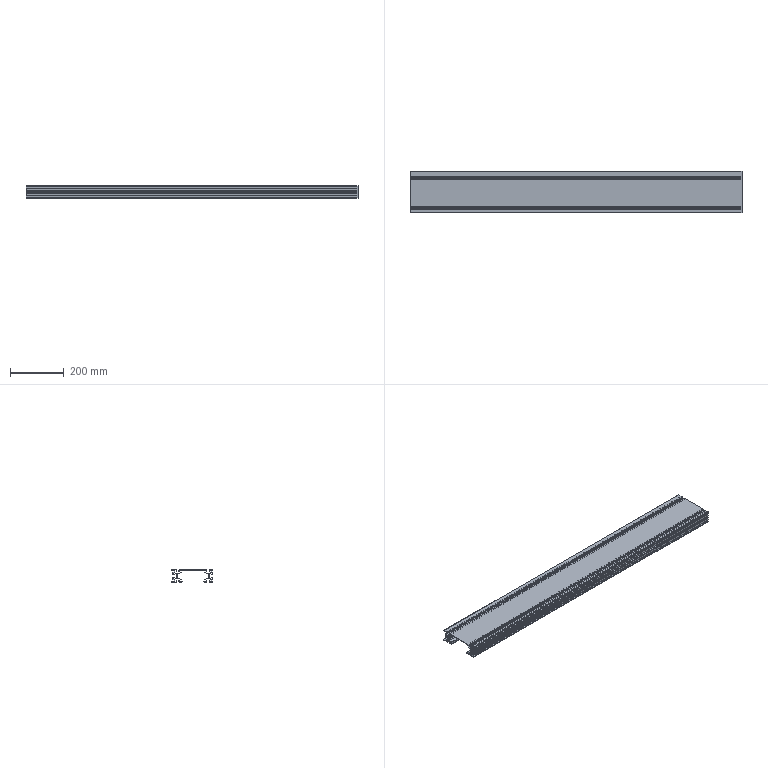Part | SolidWorks | features BaseBody 1 | 1 solid | 184 faces | box 1230 x 155 x 45 mm | volume 1472730 mm3 | plane 172 | cylinder 12 | commonest cylinder face diameters 0.4 x4 2 x4 4 x4